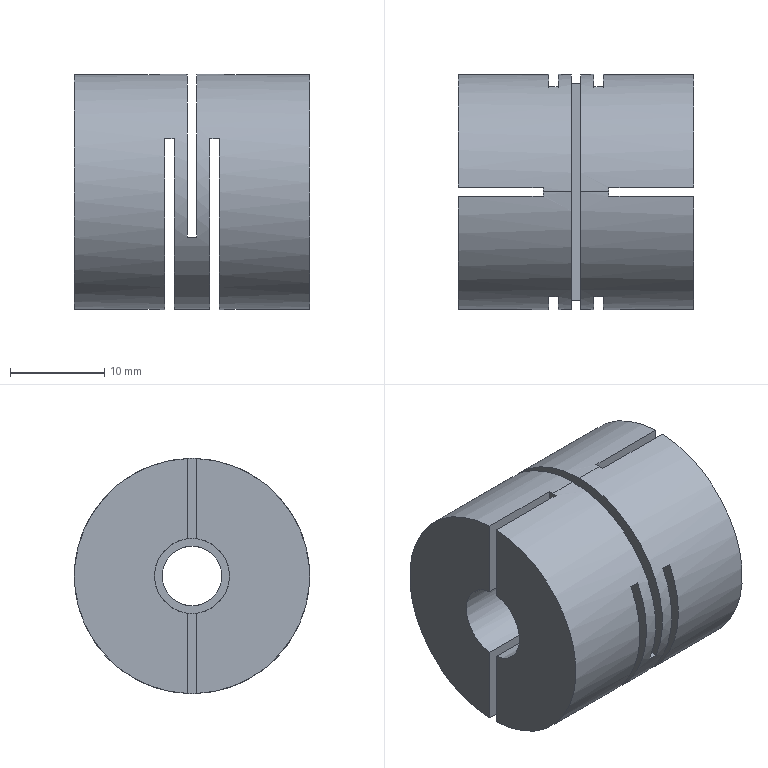Part | STEP file | Coupling CPS-φ6.35-φ8 | 1 solid | 35 faces | box 25 x 25 x 25 mm | volume 9924 mm3 | plane 25 | cylinder 10 | commonest cylinder face diameters 6.35 x4 8 x4 25 x2